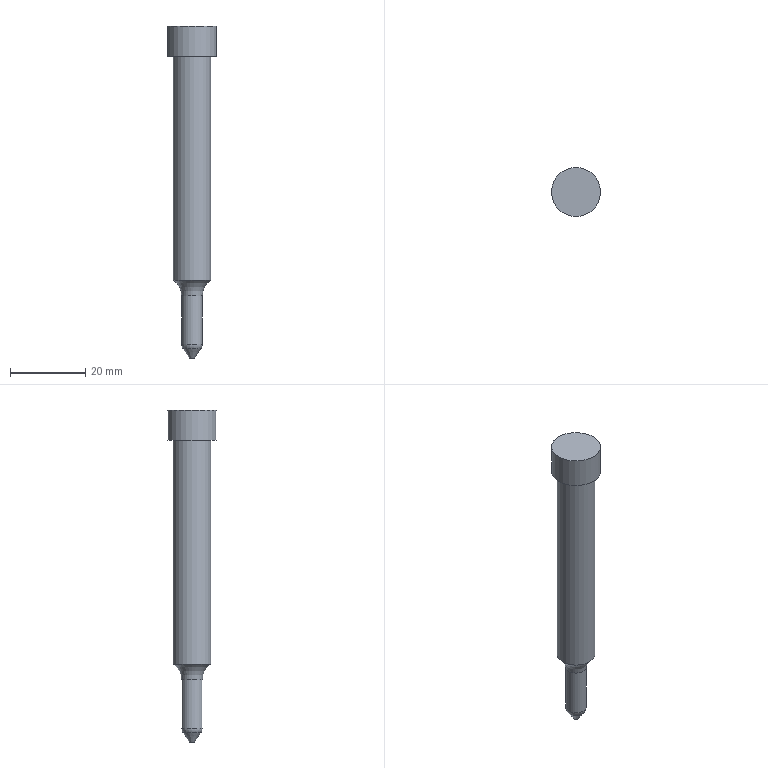Part | NX | features solid 2 | 1 solid | 9 faces | box 13 x 13 x 88 mm | volume 6239 mm3 | plane 3 | cylinder 3 | torus 2 | cone 1 | commonest cylinder face diameters 5.55 x1 10 x1 13 x1
STEP:
#1=CARTESIAN_POINT('',(3338.766,-809.537,945.716));
#2=VERTEX_POINT('',#1);
#3=CARTESIAN_POINT('',(3332.266,-809.537,945.716));
#4=DIRECTION('',(0.,0.,1.));
#5=DIRECTION('',(1.,0.,0.));
#6=AXIS2_PLACEMENT_3D('',#3,#4,#5);
#7=CIRCLE('',#6,6.5);
#8=EDGE_CURVE('',#2,#2,#7,.T.);
#9=ORIENTED_EDGE('',*,*,#8,.T.);
#10=EDGE_LOOP('',(#9));
#11=FACE_BOUND('',#10,.T.);
#12=CARTESIAN_POINT('',(2875.665,-762.453,945.716));
#13=DIRECTION('',(0.,0.,1.));
#14=DIRECTION('',(1.,0.,0.));
#15=AXIS2_PLACEMENT_3D('',#12,#13,#14);
#16=PLANE('',#15);
#17=ADVANCED_FACE('',(#11),#16,.T.);
#18=CARTESIAN_POINT('',(3338.766,-809.537,937.716));
#19=VERTEX_POINT('',#18);
#20=CARTESIAN_POINT('',(3332.266,-809.537,937.716));
#21=DIRECTION('',(0.,0.,1.));
#22=DIRECTION('',(1.,0.,0.));
#23=AXIS2_PLACEMENT_3D('',#20,#21,#22);
#24=CIRCLE('',#23,6.5);
#25=EDGE_CURVE('',#19,#19,#24,.T.);
#26=ORIENTED_EDGE('',*,*,#25,.T.);
#27=EDGE_LOOP('',(#26));
#28=FACE_BOUND('',#27,.T.);
#29=ORIENTED_EDGE('',*,*,#8,.F.);
#30=EDGE_LOOP('',(#29));
#31=FACE_BOUND('',#30,.T.);
#32=CARTESIAN_POINT('',(3332.266,-809.537,958.716));
#33=DIRECTION('',(0.,0.,-1.));
#34=DIRECTION('',(-1.,0.,0.));
#35=AXIS2_PLACEMENT_3D('',#32,#33,#34);
#36=CYLINDRICAL_SURFACE('',#35,6.5);
#37=ADVANCED_FACE('',(#28,#31),#36,.T.);
#38=CARTESIAN_POINT('',(3337.266,-809.537,937.716));
#39=VERTEX_POINT('',#38);
#40=CARTESIAN_POINT('',(3332.266,-809.537,937.716));
#41=DIRECTION('',(0.,0.,1.));
#42=DIRECTION('',(1.,0.,0.));
#43=AXIS2_PLACEMENT_3D('',#40,#41,#42);
#44=CIRCLE('',#43,5.);
#45=EDGE_CURVE('',#39,#39,#44,.F.);
#46=ORIENTED_EDGE('',*,*,#45,.F.);
#47=EDGE_LOOP('',(#46));
#48=FACE_BOUND('',#47,.T.);
#49=ORIENTED_EDGE('',*,*,#25,.F.);
#50=EDGE_LOOP('',(#49));
#51=FACE_BOUND('',#50,.T.);
#52=CARTESIAN_POINT('',(3332.266,-809.537,937.716));
#53=DIRECTION('',(0.,0.,1.));
#54=DIRECTION('',(1.,0.,0.));
#55=AXIS2_PLACEMENT_3D('',#52,#53,#54);
#56=PLANE('',#55);
#57=ADVANCED_FACE('',(#48,#51),#56,.F.);
#58=CARTESIAN_POINT('',(3327.266,-809.537,878.376));
#59=VERTEX_POINT('',#58);
#60=CARTESIAN_POINT('',(3332.266,-809.537,878.376));
#61=DIRECTION('',(0.,0.,-1.));
#62=DIRECTION('',(-1.,0.,0.));
#63=AXIS2_PLACEMENT_3D('',#60,#61,#62);
#64=CIRCLE('',#63,5.);
#65=EDGE_CURVE('',#59,#59,#64,.F.);
#66=ORIENTED_EDGE('',*,*,#65,.T.);
#67=EDGE_LOOP('',(#66));
#68=FACE_BOUND('',#67,.T.);
#69=ORIENTED_EDGE('',*,*,#45,.T.);
#70=EDGE_LOOP('',(#69));
#71=FACE_BOUND('',#70,.T.);
#72=CARTESIAN_POINT('',(3332.266,-809.537,948.716));
#73=DIRECTION('',(0.,0.,-1.));
#74=DIRECTION('',(-1.,0.,0.));
#75=AXIS2_PLACEMENT_3D('',#72,#73,#74);
#76=CYLINDRICAL_SURFACE('',#75,5.);
#77=ADVANCED_FACE('',(#68,#71),#76,.T.);
#78=CARTESIAN_POINT('',(3335.041,-809.537,874.216));
#79=VERTEX_POINT('',#78);
#80=CARTESIAN_POINT('',(3332.266,-809.537,874.216));
#81=DIRECTION('',(0.,0.,1.));
#82=DIRECTION('',(1.,0.,0.));
#83=AXIS2_PLACEMENT_3D('',#80,#81,#82);
#84=CIRCLE('',#83,2.775);
#85=EDGE_CURVE('',#79,#79,#84,.F.);
#86=ORIENTED_EDGE('',*,*,#85,.T.);
#87=EDGE_LOOP('',(#86));
#88=FACE_BOUND('',#87,.T.);
#89=CARTESIAN_POINT('',(3329.491,-809.537,861.347));
#90=VERTEX_POINT('',#89);
#91=CARTESIAN_POINT('',(3332.266,-809.537,861.347));
#92=DIRECTION('',(0.,0.,-1.));
#93=DIRECTION('',(-1.,0.,0.));
#94=AXIS2_PLACEMENT_3D('',#91,#92,#93);
#95=CIRCLE('',#94,2.775);
#96=EDGE_CURVE('',#90,#90,#95,.F.);
#97=ORIENTED_EDGE('',*,*,#96,.T.);
#98=EDGE_LOOP('',(#97));
#99=FACE_BOUND('',#98,.T.);
#100=CARTESIAN_POINT('',(3332.266,-809.537,868.716));
#101=DIRECTION('',(0.,0.,-1.));
#102=DIRECTION('',(1.,0.,0.));
#103=AXIS2_PLACEMENT_3D('',#100,#101,#102);
#104=CYLINDRICAL_SURFACE('',#103,2.775);
#105=ADVANCED_FACE('',(#88,#99),#104,.T.);
#106=CARTESIAN_POINT('',(3332.94,-809.537,857.716));
#107=VERTEX_POINT('',#106);
#108=CARTESIAN_POINT('',(3332.266,-809.537,857.716));
#109=DIRECTION('',(0.,0.,1.));
#110=DIRECTION('',(1.,0.,0.));
#111=AXIS2_PLACEMENT_3D('',#108,#109,#110);
#112=CIRCLE('',#111,0.6744);
#113=EDGE_CURVE('',#107,#107,#112,.F.);
#114=ORIENTED_EDGE('',*,*,#113,.T.);
#115=EDGE_LOOP('',(#114));
#116=FACE_BOUND('',#115,.T.);
#117=CARTESIAN_POINT('',(3332.266,-809.537,857.716));
#118=DIRECTION('',(0.,0.,1.));
#119=DIRECTION('',(1.,0.,0.));
#120=AXIS2_PLACEMENT_3D('',#117,#118,#119);
#121=PLANE('',#120);
#122=ADVANCED_FACE('',(#116),#121,.F.);
#123=CARTESIAN_POINT('',(3334.679,-809.537,860.2));
#124=VERTEX_POINT('',#123);
#125=CARTESIAN_POINT('',(3332.266,-809.537,860.2));
#126=DIRECTION('',(0.,0.,1.));
#127=DIRECTION('',(1.,0.,0.));
#128=AXIS2_PLACEMENT_3D('',#125,#126,#127);
#129=CIRCLE('',#128,2.413);
#130=EDGE_CURVE('',#124,#124,#129,.F.);
#131=ORIENTED_EDGE('',*,*,#130,.T.);
#132=EDGE_LOOP('',(#131));
#133=FACE_BOUND('',#132,.T.);
#134=ORIENTED_EDGE('',*,*,#113,.F.);
#135=EDGE_LOOP('',(#134));
#136=FACE_BOUND('',#135,.T.);
#137=CARTESIAN_POINT('',(3332.266,-809.537,860.716));
#138=DIRECTION('',(0.,0.,1.));
#139=DIRECTION('',(1.,0.,0.));
#140=AXIS2_PLACEMENT_3D('',#137,#138,#139);
#141=CONICAL_SURFACE('',#140,2.775,0.6109);
#142=ADVANCED_FACE('',(#133,#136),#141,.T.);
#143=ORIENTED_EDGE('',*,*,#130,.F.);
#144=EDGE_LOOP('',(#143));
#145=FACE_BOUND('',#144,.T.);
#146=ORIENTED_EDGE('',*,*,#96,.F.);
#147=EDGE_LOOP('',(#146));
#148=FACE_BOUND('',#147,.T.);
#149=CARTESIAN_POINT('',(3332.266,-809.537,861.347));
#150=DIRECTION('',(0.,0.,-1.));
#151=DIRECTION('',(-1.,0.,0.));
#152=AXIS2_PLACEMENT_3D('',#149,#150,#151);
#153=DEGENERATE_TOROIDAL_SURFACE('',#152,0.775,2.,.T.);
#154=ADVANCED_FACE('',(#145,#148),#153,.T.);
#155=ORIENTED_EDGE('',*,*,#85,.F.);
#156=EDGE_LOOP('',(#155));
#157=FACE_BOUND('',#156,.T.);
#158=ORIENTED_EDGE('',*,*,#65,.F.);
#159=EDGE_LOOP('',(#158));
#160=FACE_BOUND('',#159,.T.);
#161=CARTESIAN_POINT('',(3332.266,-809.537,874.216));
#162=DIRECTION('',(0.,0.,1.));
#163=DIRECTION('',(1.,0.,0.));
#164=AXIS2_PLACEMENT_3D('',#161,#162,#163);
#165=TOROIDAL_SURFACE('',#164,7.775,5.);
#166=ADVANCED_FACE('',(#157,#160),#165,.F.);
#167=CLOSED_SHELL('',(#17,#37,#57,#77,#105,#122,#142,#154,#166));
#168=MANIFOLD_SOLID_BREP('',#167);
#169=(LENGTH_UNIT()NAMED_UNIT(*)SI_UNIT(.MILLI.,.METRE.));
#170=UNCERTAINTY_MEASURE_WITH_UNIT(LENGTH_MEASURE(0.00001),#169,'','');
#171=(NAMED_UNIT(*)PLANE_ANGLE_UNIT()SI_UNIT($,.RADIAN.));
#172=(NAMED_UNIT(*)SI_UNIT($,.STERADIAN.)SOLID_ANGLE_UNIT());
#173=(GEOMETRIC_REPRESENTATION_CONTEXT(3)GLOBAL_UNCERTAINTY_ASSIGNED_CONTEXT((#170))GLOBAL_UNIT_ASSIGNED_CONTEXT((#169,#171,#172))REPRESENTATION_CONTEXT('',''));
#174=ADVANCED_BREP_SHAPE_REPRESENTATION('',(#168),#173);